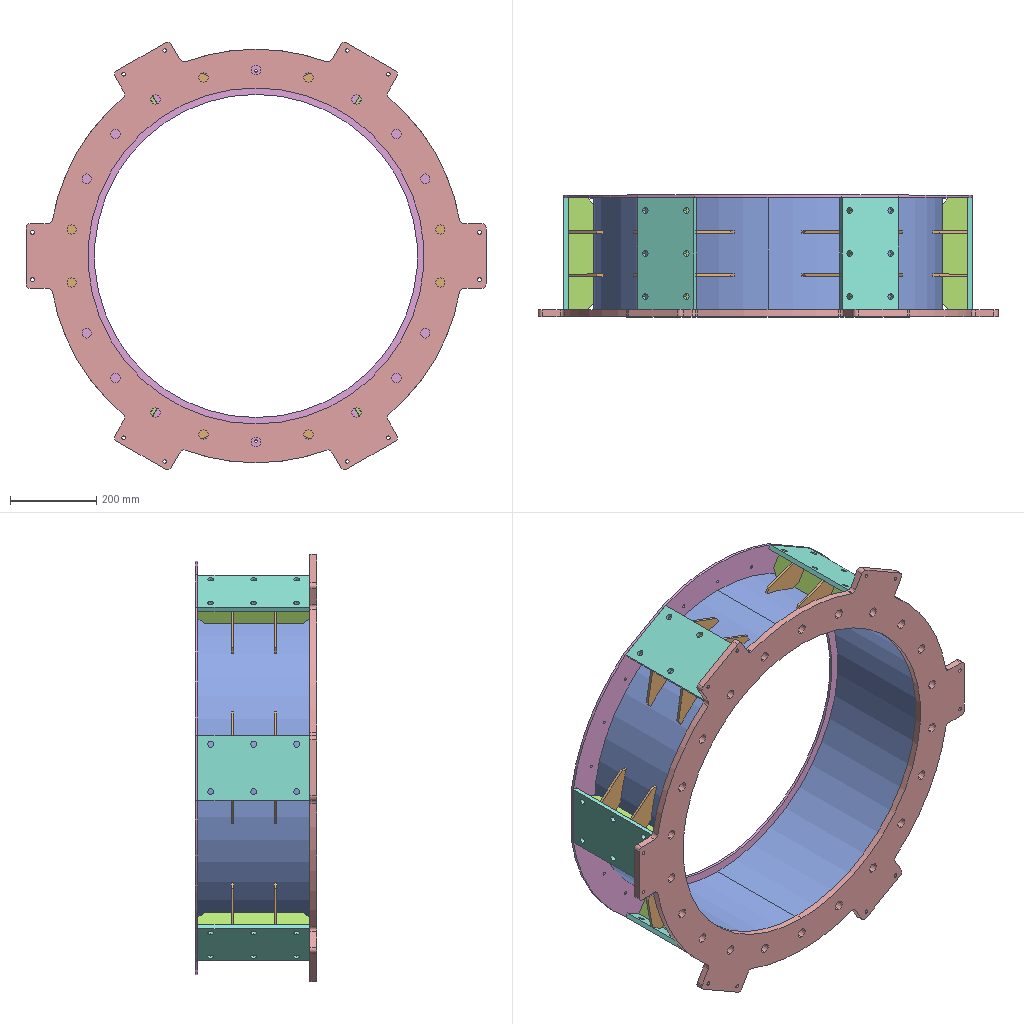Assembly | SolidWorks | 6 different items | 45 placed | box 1068 x 282 x 993 mm
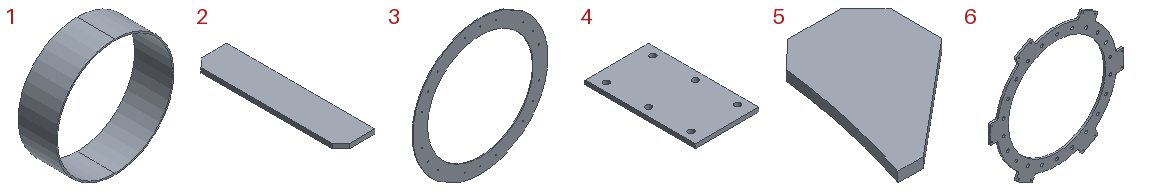Parts list (item | quantity | size | volume | features):
1 | x1 | 810 x 260 x 810 mm | 6534513 mm3 | features Extrusion 1
2 | x12 | 60 x 260 x 8 mm | 123000 mm3 | features Chamfer 1, Extrusion 1
3 | x1 | 948 x 6 x 960 mm | 1666480 mm3 | features CirPattern 1, Extrusion 1, HoleWzd 1, ICE 1
4 | x6 | 150 x 260 x 10 mm | 380764 mm3 | features Extrusion 1, HoleWzd 1
5 | x24 | 81 x 100 x 6 mm | 28941 mm3 | features Extrusion 1
6 | x1 | 1068 x 16 x 992.595 mm | 4595541 mm3 | features HoleWzd 2, Extrusion 1, Fillet 1
Mates (type | each side: item.copy, entity, surface, feature):
Concentric | 6.1 face cylinder Boss-Extrude1 | 1.1 face cylinder Boss-Extrude1
Coincident | 6.1 face plane Boss-Extrude1 | 1.1 face plane Boss-Extrude1
Concentric | 1.1 face cylinder Boss-Extrude1 | 3.1 face cylinder Boss-Extrude1
Coincident | 1.1 face plane Boss-Extrude1 | 3.1 face plane Boss-Extrude1
Parallel | 6.1 face plane Boss-Extrude1 | 3.1 face plane Cut-Extrude3
Coincident | 3.1 face plane Cut-Extrude3 | 4.1 face plane Boss-Extrude1
Coincident | 3.1 face plane Boss-Extrude1 | 4.1 face plane Boss-Extrude1
Coincident | 6.1 face plane Boss-Extrude1 | 4.1 face plane Boss-Extrude1
Coincident | 2.1 face plane Boss-Extrude1 | 2.2 face plane Boss-Extrude1 | 2 times
DistanceDim | 2.1 face plane Boss-Extrude1 | 2.2 face plane Boss-Extrude1
Coincident | 6.1 face plane Boss-Extrude1 | 2.1 face plane Boss-Extrude1
Coincident | 2.1 face plane Boss-Extrude1 | 4.1 face plane Boss-Extrude1
Width | 4.1 face plane Boss-Extrude1 | 4.1 face plane Boss-Extrude1 | 2.1 face plane Boss-Extrude1 | 2.2 face plane Boss-Extrude1
Coincident | 4.1 face plane Boss-Extrude1 | 5.1 face plane Boss-Extrude1
Coincident | 2.1 face plane Boss-Extrude1 | 5.1 face plane Boss-Extrude1
Coincident | 2.1 face plane Boss-Extrude1 | 5.2 face plane Boss-Extrude1
Coincident | 4.1 face plane Boss-Extrude1 | 5.2 face plane Boss-Extrude1
DistanceDim | 5.1 face plane Boss-Extrude1 | 3.1 face plane Boss-Extrude1
DistanceDim | 5.2 face plane Boss-Extrude1 | 5.1 face plane Boss-Extrude1